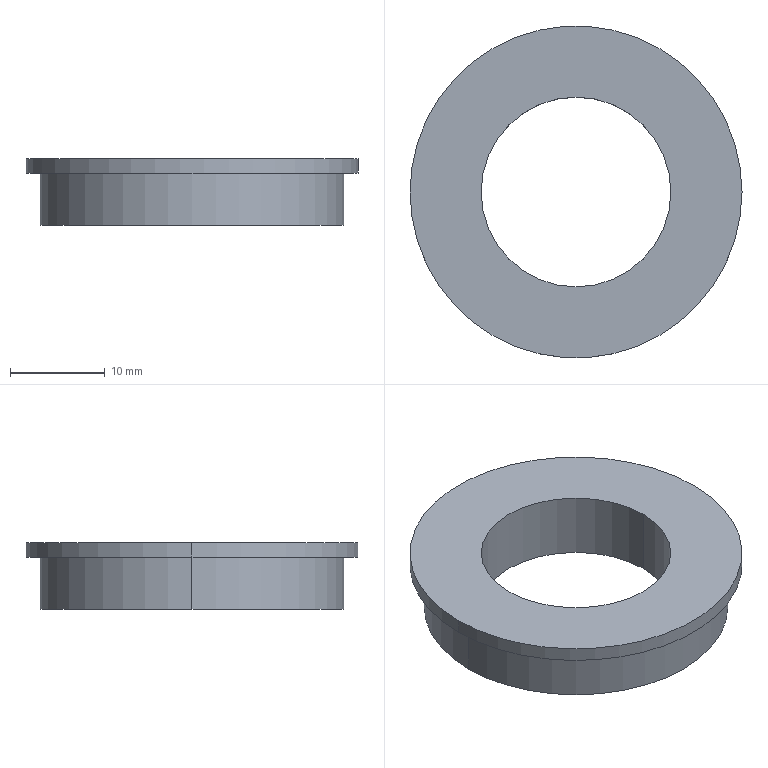Part | SolidWorks | features Extrusion 1, ICE 1 | 1 solid | 9 faces | box 35 x 35 x 7 mm | volume 3667 mm3 | cylinder 6 | plane 3 | commonest cylinder face diameters 20 x2 32 x2 35 x2
STEP:
#1=CARTESIAN_POINT('',(17.5,0.,5.5));
#2=VERTEX_POINT('',#1);
#3=CARTESIAN_POINT('',(-17.5,0.,5.5));
#4=VERTEX_POINT('',#3);
#5=CARTESIAN_POINT('',(0.,0.,5.5));
#6=DIRECTION('',(0.,0.,1.));
#7=DIRECTION('',(1.,0.,0.));
#8=AXIS2_PLACEMENT_3D('',#5,#6,#7);
#9=CIRCLE('',#8,17.5);
#10=EDGE_CURVE('',#2,#4,#9,.T.);
#11=ORIENTED_EDGE('',*,*,#10,.T.);
#12=CARTESIAN_POINT('',(-17.5,0.,7.));
#13=VERTEX_POINT('',#12);
#14=CARTESIAN_POINT('',(-17.5,0.,5.5));
#15=DIRECTION('',(0.,0.,1.));
#16=VECTOR('',#15,1000.);
#17=LINE('',#14,#16);
#18=EDGE_CURVE('',#4,#13,#17,.T.);
#19=ORIENTED_EDGE('',*,*,#18,.T.);
#20=CARTESIAN_POINT('',(17.5,0.,7.));
#21=VERTEX_POINT('',#20);
#22=CARTESIAN_POINT('',(0.,0.,7.));
#23=DIRECTION('',(0.,0.,1.));
#24=DIRECTION('',(1.,0.,0.));
#25=AXIS2_PLACEMENT_3D('',#22,#23,#24);
#26=CIRCLE('',#25,17.5);
#27=EDGE_CURVE('',#21,#13,#26,.T.);
#28=ORIENTED_EDGE('',*,*,#27,.F.);
#29=CARTESIAN_POINT('',(17.5,0.,5.5));
#30=DIRECTION('',(0.,0.,1.));
#31=VECTOR('',#30,1000.);
#32=LINE('',#29,#31);
#33=EDGE_CURVE('',#2,#21,#32,.T.);
#34=ORIENTED_EDGE('',*,*,#33,.F.);
#35=EDGE_LOOP('',(#11,#19,#28,#34));
#36=FACE_OUTER_BOUND('',#35,.T.);
#37=CARTESIAN_POINT('',(0.,0.,5.5));
#38=DIRECTION('',(0.,0.,1.));
#39=DIRECTION('',(1.,0.,0.));
#40=AXIS2_PLACEMENT_3D('',#37,#38,#39);
#41=CYLINDRICAL_SURFACE('',#40,17.5);
#42=ADVANCED_FACE('',(#36),#41,.T.);
#43=CARTESIAN_POINT('',(-10.,0.,7.));
#44=VERTEX_POINT('',#43);
#45=CARTESIAN_POINT('',(10.,0.,7.));
#46=VERTEX_POINT('',#45);
#47=CARTESIAN_POINT('',(0.,0.,7.));
#48=DIRECTION('',(0.,0.,1.));
#49=DIRECTION('',(1.,0.,0.));
#50=AXIS2_PLACEMENT_3D('',#47,#48,#49);
#51=CIRCLE('',#50,10.);
#52=EDGE_CURVE('',#44,#46,#51,.T.);
#53=ORIENTED_EDGE('',*,*,#52,.T.);
#54=CARTESIAN_POINT('',(10.,0.,0.));
#55=VERTEX_POINT('',#54);
#56=CARTESIAN_POINT('',(10.,0.,7.));
#57=DIRECTION('',(0.,0.,-1.));
#58=VECTOR('',#57,1000.);
#59=LINE('',#56,#58);
#60=EDGE_CURVE('',#46,#55,#59,.T.);
#61=ORIENTED_EDGE('',*,*,#60,.T.);
#62=CARTESIAN_POINT('',(-10.,0.,0.));
#63=VERTEX_POINT('',#62);
#64=CARTESIAN_POINT('',(0.,0.,0.));
#65=DIRECTION('',(0.,0.,1.));
#66=DIRECTION('',(1.,0.,0.));
#67=AXIS2_PLACEMENT_3D('',#64,#65,#66);
#68=CIRCLE('',#67,10.);
#69=EDGE_CURVE('',#63,#55,#68,.T.);
#70=ORIENTED_EDGE('',*,*,#69,.F.);
#71=CARTESIAN_POINT('',(-10.,0.,7.));
#72=DIRECTION('',(0.,0.,-1.));
#73=VECTOR('',#72,1000.);
#74=LINE('',#71,#73);
#75=EDGE_CURVE('',#44,#63,#74,.T.);
#76=ORIENTED_EDGE('',*,*,#75,.F.);
#77=EDGE_LOOP('',(#53,#61,#70,#76));
#78=FACE_OUTER_BOUND('',#77,.T.);
#79=CARTESIAN_POINT('',(0.,0.,7.));
#80=DIRECTION('',(0.,0.,-1.));
#81=DIRECTION('',(-1.,0.,0.));
#82=AXIS2_PLACEMENT_3D('',#79,#80,#81);
#83=CYLINDRICAL_SURFACE('',#82,10.);
#84=ADVANCED_FACE('',(#78),#83,.F.);
#85=CARTESIAN_POINT('',(16.,0.,5.5));
#86=VERTEX_POINT('',#85);
#87=CARTESIAN_POINT('',(-16.,0.,5.5));
#88=VERTEX_POINT('',#87);
#89=CARTESIAN_POINT('',(0.,0.,5.5));
#90=DIRECTION('',(0.,0.,1.));
#91=DIRECTION('',(1.,0.,0.));
#92=AXIS2_PLACEMENT_3D('',#89,#90,#91);
#93=CIRCLE('',#92,16.);
#94=EDGE_CURVE('',#86,#88,#93,.T.);
#95=ORIENTED_EDGE('',*,*,#94,.F.);
#96=CARTESIAN_POINT('',(16.,0.,0.));
#97=VERTEX_POINT('',#96);
#98=CARTESIAN_POINT('',(16.,0.,7.));
#99=DIRECTION('',(0.,0.,-1.));
#100=VECTOR('',#99,1000.);
#101=LINE('',#98,#100);
#102=EDGE_CURVE('',#86,#97,#101,.T.);
#103=ORIENTED_EDGE('',*,*,#102,.T.);
#104=CARTESIAN_POINT('',(-16.,0.,0.));
#105=VERTEX_POINT('',#104);
#106=CARTESIAN_POINT('',(0.,0.,0.));
#107=DIRECTION('',(0.,0.,1.));
#108=DIRECTION('',(1.,0.,0.));
#109=AXIS2_PLACEMENT_3D('',#106,#107,#108);
#110=CIRCLE('',#109,16.);
#111=EDGE_CURVE('',#97,#105,#110,.T.);
#112=ORIENTED_EDGE('',*,*,#111,.T.);
#113=CARTESIAN_POINT('',(-16.,0.,7.));
#114=DIRECTION('',(0.,0.,-1.));
#115=VECTOR('',#114,1000.);
#116=LINE('',#113,#115);
#117=EDGE_CURVE('',#88,#105,#116,.T.);
#118=ORIENTED_EDGE('',*,*,#117,.F.);
#119=EDGE_LOOP('',(#95,#103,#112,#118));
#120=FACE_OUTER_BOUND('',#119,.T.);
#121=CARTESIAN_POINT('',(0.,0.,7.));
#122=DIRECTION('',(0.,0.,-1.));
#123=DIRECTION('',(-1.,0.,0.));
#124=AXIS2_PLACEMENT_3D('',#121,#122,#123);
#125=CYLINDRICAL_SURFACE('',#124,16.);
#126=ADVANCED_FACE('',(#120),#125,.T.);
#127=ORIENTED_EDGE('',*,*,#102,.F.);
#128=CARTESIAN_POINT('',(0.,0.,5.5));
#129=DIRECTION('',(0.,0.,1.));
#130=DIRECTION('',(1.,0.,0.));
#131=AXIS2_PLACEMENT_3D('',#128,#129,#130);
#132=CIRCLE('',#131,16.);
#133=EDGE_CURVE('',#88,#86,#132,.T.);
#134=ORIENTED_EDGE('',*,*,#133,.F.);
#135=ORIENTED_EDGE('',*,*,#117,.T.);
#136=CARTESIAN_POINT('',(0.,0.,0.));
#137=DIRECTION('',(0.,0.,1.));
#138=DIRECTION('',(1.,0.,0.));
#139=AXIS2_PLACEMENT_3D('',#136,#137,#138);
#140=CIRCLE('',#139,16.);
#141=EDGE_CURVE('',#105,#97,#140,.T.);
#142=ORIENTED_EDGE('',*,*,#141,.T.);
#143=EDGE_LOOP('',(#127,#134,#135,#142));
#144=FACE_OUTER_BOUND('',#143,.T.);
#145=CARTESIAN_POINT('',(0.,0.,7.));
#146=DIRECTION('',(0.,0.,-1.));
#147=DIRECTION('',(-1.,0.,0.));
#148=AXIS2_PLACEMENT_3D('',#145,#146,#147);
#149=CYLINDRICAL_SURFACE('',#148,16.);
#150=ADVANCED_FACE('',(#144),#149,.T.);
#151=ORIENTED_EDGE('',*,*,#52,.F.);
#152=CARTESIAN_POINT('',(0.,0.,7.));
#153=DIRECTION('',(0.,0.,1.));
#154=DIRECTION('',(1.,0.,0.));
#155=AXIS2_PLACEMENT_3D('',#152,#153,#154);
#156=CIRCLE('',#155,10.);
#157=EDGE_CURVE('',#46,#44,#156,.T.);
#158=ORIENTED_EDGE('',*,*,#157,.F.);
#159=EDGE_LOOP('',(#151,#158));
#160=FACE_BOUND('',#159,.T.);
#161=ORIENTED_EDGE('',*,*,#27,.T.);
#162=CARTESIAN_POINT('',(0.,0.,7.));
#163=DIRECTION('',(0.,0.,1.));
#164=DIRECTION('',(1.,0.,0.));
#165=AXIS2_PLACEMENT_3D('',#162,#163,#164);
#166=CIRCLE('',#165,17.5);
#167=EDGE_CURVE('',#13,#21,#166,.T.);
#168=ORIENTED_EDGE('',*,*,#167,.T.);
#169=EDGE_LOOP('',(#161,#168));
#170=FACE_OUTER_BOUND('',#169,.T.);
#171=CARTESIAN_POINT('',(0.,0.,7.));
#172=DIRECTION('',(0.,0.,1.));
#173=DIRECTION('',(1.,0.,0.));
#174=AXIS2_PLACEMENT_3D('',#171,#172,#173);
#175=PLANE('',#174);
#176=ADVANCED_FACE('',(#160,#170),#175,.T.);
#177=ORIENTED_EDGE('',*,*,#141,.F.);
#178=ORIENTED_EDGE('',*,*,#111,.F.);
#179=EDGE_LOOP('',(#177,#178));
#180=FACE_OUTER_BOUND('',#179,.T.);
#181=ORIENTED_EDGE('',*,*,#69,.T.);
#182=CARTESIAN_POINT('',(0.,0.,0.));
#183=DIRECTION('',(0.,0.,1.));
#184=DIRECTION('',(1.,0.,0.));
#185=AXIS2_PLACEMENT_3D('',#182,#183,#184);
#186=CIRCLE('',#185,10.);
#187=EDGE_CURVE('',#55,#63,#186,.T.);
#188=ORIENTED_EDGE('',*,*,#187,.T.);
#189=EDGE_LOOP('',(#181,#188));
#190=FACE_BOUND('',#189,.T.);
#191=CARTESIAN_POINT('',(0.,0.,0.));
#192=DIRECTION('',(0.,0.,1.));
#193=DIRECTION('',(1.,0.,0.));
#194=AXIS2_PLACEMENT_3D('',#191,#192,#193);
#195=PLANE('',#194);
#196=ADVANCED_FACE('',(#180,#190),#195,.F.);
#197=ORIENTED_EDGE('',*,*,#60,.F.);
#198=ORIENTED_EDGE('',*,*,#157,.T.);
#199=ORIENTED_EDGE('',*,*,#75,.T.);
#200=ORIENTED_EDGE('',*,*,#187,.F.);
#201=EDGE_LOOP('',(#197,#198,#199,#200));
#202=FACE_OUTER_BOUND('',#201,.T.);
#203=CARTESIAN_POINT('',(0.,0.,7.));
#204=DIRECTION('',(0.,0.,-1.));
#205=DIRECTION('',(-1.,0.,0.));
#206=AXIS2_PLACEMENT_3D('',#203,#204,#205);
#207=CYLINDRICAL_SURFACE('',#206,10.);
#208=ADVANCED_FACE('',(#202),#207,.F.);
#209=ORIENTED_EDGE('',*,*,#18,.F.);
#210=CARTESIAN_POINT('',(0.,0.,5.5));
#211=DIRECTION('',(0.,0.,1.));
#212=DIRECTION('',(1.,0.,0.));
#213=AXIS2_PLACEMENT_3D('',#210,#211,#212);
#214=CIRCLE('',#213,17.5);
#215=EDGE_CURVE('',#4,#2,#214,.T.);
#216=ORIENTED_EDGE('',*,*,#215,.T.);
#217=ORIENTED_EDGE('',*,*,#33,.T.);
#218=ORIENTED_EDGE('',*,*,#167,.F.);
#219=EDGE_LOOP('',(#209,#216,#217,#218));
#220=FACE_OUTER_BOUND('',#219,.T.);
#221=CARTESIAN_POINT('',(0.,0.,5.5));
#222=DIRECTION('',(0.,0.,1.));
#223=DIRECTION('',(1.,0.,0.));
#224=AXIS2_PLACEMENT_3D('',#221,#222,#223);
#225=CYLINDRICAL_SURFACE('',#224,17.5);
#226=ADVANCED_FACE('',(#220),#225,.T.);
#227=ORIENTED_EDGE('',*,*,#133,.T.);
#228=ORIENTED_EDGE('',*,*,#94,.T.);
#229=EDGE_LOOP('',(#227,#228));
#230=FACE_BOUND('',#229,.T.);
#231=ORIENTED_EDGE('',*,*,#10,.F.);
#232=ORIENTED_EDGE('',*,*,#215,.F.);
#233=EDGE_LOOP('',(#231,#232));
#234=FACE_OUTER_BOUND('',#233,.T.);
#235=CARTESIAN_POINT('',(0.,0.,5.5));
#236=DIRECTION('',(0.,0.,1.));
#237=DIRECTION('',(1.,0.,0.));
#238=AXIS2_PLACEMENT_3D('',#235,#236,#237);
#239=PLANE('',#238);
#240=ADVANCED_FACE('',(#230,#234),#239,.F.);
#241=CLOSED_SHELL('',(#42,#84,#126,#150,#176,#196,#208,#226,#240));
#242=MANIFOLD_SOLID_BREP('',#241);
#243=CARTESIAN_POINT('',(0.,0.,0.));
#244=DIRECTION('',(0.,0.,1.));
#245=DIRECTION('',(1.,0.,0.));
#246=AXIS2_PLACEMENT_3D('',#243,#244,#245);
#247=(LENGTH_UNIT()NAMED_UNIT(*)SI_UNIT(.MILLI.,.METRE.));
#248=UNCERTAINTY_MEASURE_WITH_UNIT(LENGTH_MEASURE(0.00001),#247,'','');
#249=(NAMED_UNIT(*)PLANE_ANGLE_UNIT()SI_UNIT($,.RADIAN.));
#250=(NAMED_UNIT(*)SI_UNIT($,.STERADIAN.)SOLID_ANGLE_UNIT());
#251=(GEOMETRIC_REPRESENTATION_CONTEXT(3)GLOBAL_UNCERTAINTY_ASSIGNED_CONTEXT((#248))GLOBAL_UNIT_ASSIGNED_CONTEXT((#247,#249,#250))REPRESENTATION_CONTEXT('',''));
#252=ADVANCED_BREP_SHAPE_REPRESENTATION('',(#242,#246),#251);